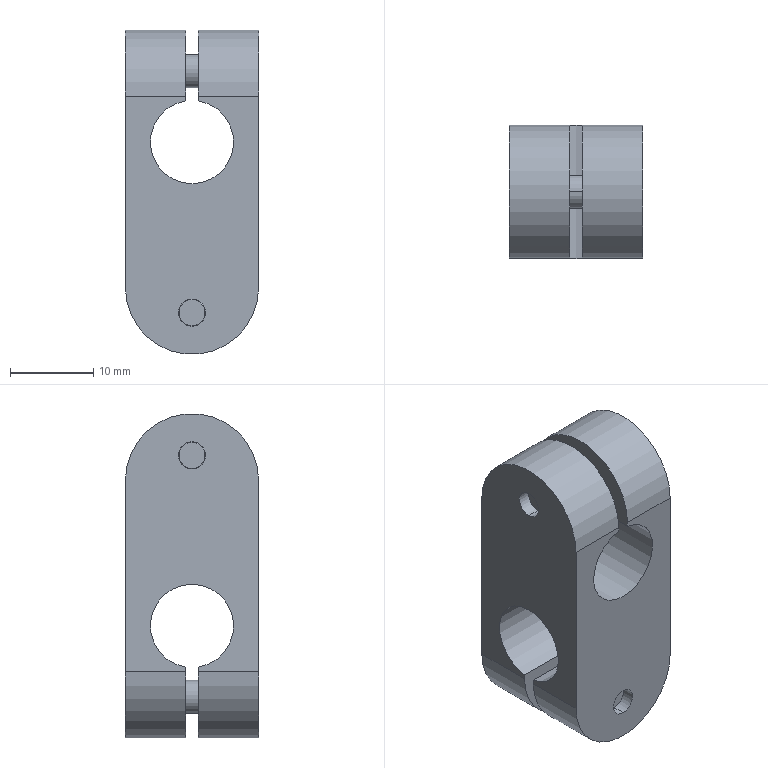Part | STEP file | Ultra-simple post clamp ALKW10 | 1 solid | 78 faces | box 16 x 16 x 39 mm | volume 6075 mm3 | plane 40 | cylinder 26 | cone 12 | commonest cylinder face diameters 3.242 x4 4 x4 4.5 x4 7 x4 8 x4 16 x4